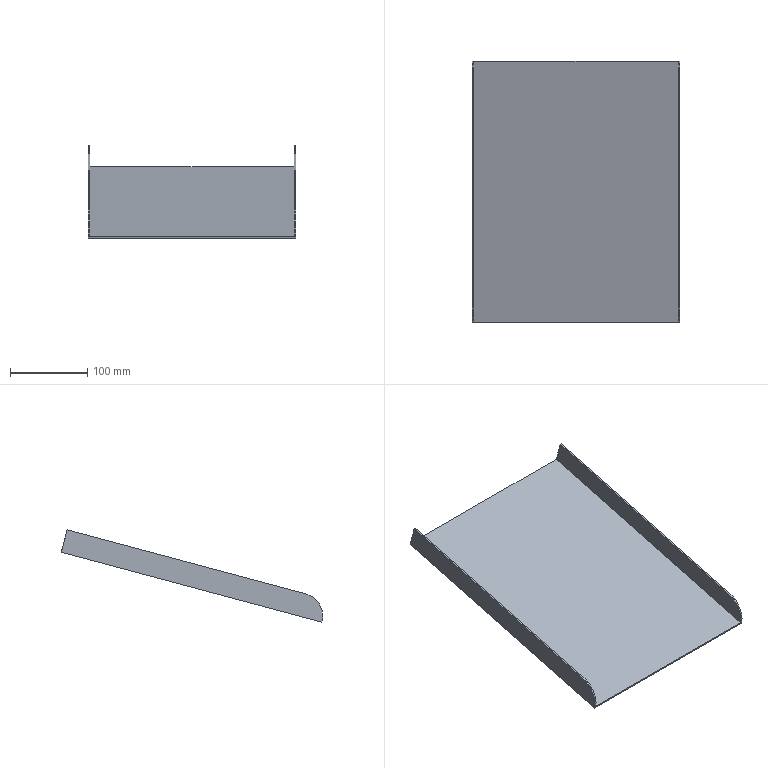Part | NX | features solid 2 | 1 solid | 12 faces | box 269.608 x 339.096 x 119.564 mm | volume 227153 mm3 | plane 10 | cylinder 2 | commonest cylinder face diameters 60 x2
STEP:
#1=CARTESIAN_POINT('',(378.,-610.733,-503.089));
#2=VERTEX_POINT('',#1);
#3=CARTESIAN_POINT('',(378.,-948.742,-593.658));
#4=VERTEX_POINT('',#3);
#5=CARTESIAN_POINT('',(378.,-784.599,-549.676));
#6=DIRECTION('',(0.,-0.9659,-0.2588));
#7=VECTOR('',#6,1000.);
#8=LINE('',#5,#7);
#9=EDGE_CURVE('',#2,#4,#8,.T.);
#10=ORIENTED_EDGE('',*,*,#9,.F.);
#11=CARTESIAN_POINT('',(112.392,-610.733,-503.089));
#12=VERTEX_POINT('',#11);
#13=CARTESIAN_POINT('',(378.,-610.733,-503.089));
#14=DIRECTION('',(1.,0.,0.));
#15=VECTOR('',#14,1000.);
#16=LINE('',#13,#15);
#17=EDGE_CURVE('',#2,#12,#16,.F.);
#18=ORIENTED_EDGE('',*,*,#17,.T.);
#19=CARTESIAN_POINT('',(112.392,-948.742,-593.658));
#20=VERTEX_POINT('',#19);
#21=CARTESIAN_POINT('',(112.392,-766.757,-544.895));
#22=DIRECTION('',(0.,0.9659,0.2588));
#23=VECTOR('',#22,1000.);
#24=LINE('',#21,#23);
#25=EDGE_CURVE('',#12,#20,#24,.F.);
#26=ORIENTED_EDGE('',*,*,#25,.T.);
#27=CARTESIAN_POINT('',(110.392,-948.742,-593.658));
#28=VERTEX_POINT('',#27);
#29=CARTESIAN_POINT('',(154.206,-948.742,-593.658));
#30=DIRECTION('',(-1.,0.,0.));
#31=VECTOR('',#30,1000.);
#32=LINE('',#29,#31);
#33=EDGE_CURVE('',#28,#20,#32,.F.);
#34=ORIENTED_EDGE('',*,*,#33,.F.);
#35=CARTESIAN_POINT('',(110.392,-948.807,-593.675));
#36=VERTEX_POINT('',#35);
#37=CARTESIAN_POINT('',(110.392,-795.624,-552.63));
#38=DIRECTION('',(0.,0.9659,0.2588));
#39=VECTOR('',#38,1000.);
#40=LINE('',#37,#39);
#41=EDGE_CURVE('',#28,#36,#40,.F.);
#42=ORIENTED_EDGE('',*,*,#41,.T.);
#43=CARTESIAN_POINT('',(380.,-948.807,-593.675));
#44=VERTEX_POINT('',#43);
#45=CARTESIAN_POINT('',(378.,-948.807,-593.675));
#46=DIRECTION('',(1.,0.,0.));
#47=VECTOR('',#46,1000.);
#48=LINE('',#45,#47);
#49=EDGE_CURVE('',#44,#36,#48,.F.);
#50=ORIENTED_EDGE('',*,*,#49,.F.);
#51=CARTESIAN_POINT('',(380.,-948.742,-593.658));
#52=VERTEX_POINT('',#51);
#53=CARTESIAN_POINT('',(380.,-784.599,-549.676));
#54=DIRECTION('',(0.,-0.9659,-0.2588));
#55=VECTOR('',#54,1000.);
#56=LINE('',#53,#55);
#57=EDGE_CURVE('',#52,#44,#56,.T.);
#58=ORIENTED_EDGE('',*,*,#57,.F.);
#59=CARTESIAN_POINT('',(390.,-948.742,-593.658));
#60=DIRECTION('',(1.,0.,0.));
#61=VECTOR('',#60,1000.);
#62=LINE('',#59,#61);
#63=EDGE_CURVE('',#4,#52,#62,.T.);
#64=ORIENTED_EDGE('',*,*,#63,.F.);
#65=EDGE_LOOP('',(#10,#18,#26,#34,#42,#50,#58,#64));
#66=FACE_BOUND('',#65,.T.);
#67=CARTESIAN_POINT('',(378.,-784.599,-549.676));
#68=DIRECTION('',(0.,-0.2588,0.9659));
#69=DIRECTION('',(1.,0.,0.));
#70=AXIS2_PLACEMENT_3D('',#67,#68,#69);
#71=PLANE('',#70);
#72=ADVANCED_FACE('',(#66),#71,.T.);
#73=ORIENTED_EDGE('',*,*,#17,.F.);
#74=CARTESIAN_POINT('',(378.,-617.98,-476.043));
#75=VERTEX_POINT('',#74);
#76=CARTESIAN_POINT('',(378.,-610.215,-505.021));
#77=DIRECTION('',(0.,0.2588,-0.9659));
#78=VECTOR('',#77,1000.);
#79=LINE('',#76,#78);
#80=EDGE_CURVE('',#2,#75,#79,.F.);
#81=ORIENTED_EDGE('',*,*,#80,.T.);
#82=CARTESIAN_POINT('',(380.,-617.98,-476.043));
#83=VERTEX_POINT('',#82);
#84=CARTESIAN_POINT('',(378.,-617.98,-476.043));
#85=DIRECTION('',(-1.,0.,0.));
#86=VECTOR('',#85,1000.);
#87=LINE('',#84,#86);
#88=EDGE_CURVE('',#83,#75,#87,.T.);
#89=ORIENTED_EDGE('',*,*,#88,.F.);
#90=CARTESIAN_POINT('',(380.,-610.215,-505.021));
#91=VERTEX_POINT('',#90);
#92=CARTESIAN_POINT('',(380.,-610.215,-505.021));
#93=DIRECTION('',(0.,0.2588,-0.9659));
#94=VECTOR('',#93,1000.);
#95=LINE('',#92,#94);
#96=EDGE_CURVE('',#91,#83,#95,.F.);
#97=ORIENTED_EDGE('',*,*,#96,.F.);
#98=CARTESIAN_POINT('',(110.392,-610.215,-505.021));
#99=VERTEX_POINT('',#98);
#100=CARTESIAN_POINT('',(378.,-610.215,-505.021));
#101=DIRECTION('',(1.,0.,0.));
#102=VECTOR('',#101,1000.);
#103=LINE('',#100,#102);
#104=EDGE_CURVE('',#91,#99,#103,.F.);
#105=ORIENTED_EDGE('',*,*,#104,.T.);
#106=CARTESIAN_POINT('',(110.392,-617.98,-476.043));
#107=VERTEX_POINT('',#106);
#108=CARTESIAN_POINT('',(110.392,-610.215,-505.021));
#109=DIRECTION('',(0.,-0.2588,0.9659));
#110=VECTOR('',#109,1000.);
#111=LINE('',#108,#110);
#112=EDGE_CURVE('',#99,#107,#111,.T.);
#113=ORIENTED_EDGE('',*,*,#112,.T.);
#114=CARTESIAN_POINT('',(112.392,-617.98,-476.043));
#115=VERTEX_POINT('',#114);
#116=CARTESIAN_POINT('',(378.,-617.98,-476.043));
#117=DIRECTION('',(-1.,0.,0.));
#118=VECTOR('',#117,1000.);
#119=LINE('',#116,#118);
#120=EDGE_CURVE('',#107,#115,#119,.F.);
#121=ORIENTED_EDGE('',*,*,#120,.T.);
#122=CARTESIAN_POINT('',(112.392,-610.215,-505.021));
#123=DIRECTION('',(0.,-0.2588,0.9659));
#124=VECTOR('',#123,1000.);
#125=LINE('',#122,#124);
#126=EDGE_CURVE('',#12,#115,#125,.T.);
#127=ORIENTED_EDGE('',*,*,#126,.F.);
#128=EDGE_LOOP('',(#73,#81,#89,#97,#105,#113,#121,#127));
#129=FACE_BOUND('',#128,.T.);
#130=CARTESIAN_POINT('',(378.,-610.215,-505.021));
#131=DIRECTION('',(0.,0.9659,0.2588));
#132=DIRECTION('',(-1.,0.,0.));
#133=AXIS2_PLACEMENT_3D('',#130,#131,#132);
#134=PLANE('',#133);
#135=ADVANCED_FACE('',(#129),#134,.T.);
#136=CARTESIAN_POINT('',(380.,-948.289,-595.607));
#137=VERTEX_POINT('',#136);
#138=CARTESIAN_POINT('',(380.,-948.289,-595.607));
#139=DIRECTION('',(0.,-0.2588,0.9659));
#140=VECTOR('',#139,1000.);
#141=LINE('',#138,#140);
#142=EDGE_CURVE('',#137,#44,#141,.T.);
#143=ORIENTED_EDGE('',*,*,#142,.F.);
#144=CARTESIAN_POINT('',(380.,-784.082,-551.608));
#145=DIRECTION('',(0.,-0.9659,-0.2588));
#146=VECTOR('',#145,1000.);
#147=LINE('',#144,#146);
#148=EDGE_CURVE('',#91,#137,#147,.T.);
#149=ORIENTED_EDGE('',*,*,#148,.F.);
#150=ORIENTED_EDGE('',*,*,#96,.T.);
#151=CARTESIAN_POINT('',(380.,-927.076,-558.865));
#152=VERTEX_POINT('',#151);
#153=CARTESIAN_POINT('',(380.,-791.846,-522.63));
#154=DIRECTION('',(0.,0.9659,0.2588));
#155=VECTOR('',#154,1000.);
#156=LINE('',#153,#155);
#157=EDGE_CURVE('',#83,#152,#156,.F.);
#158=ORIENTED_EDGE('',*,*,#157,.T.);
#159=CARTESIAN_POINT('',(380.,-919.311,-587.843));
#160=DIRECTION('',(-1.,0.,0.));
#161=DIRECTION('',(0.,0.,1.));
#162=AXIS2_PLACEMENT_3D('',#159,#160,#161);
#163=CIRCLE('',#162,30.);
#164=EDGE_CURVE('',#152,#52,#163,.F.);
#165=ORIENTED_EDGE('',*,*,#164,.T.);
#166=ORIENTED_EDGE('',*,*,#57,.T.);
#167=EDGE_LOOP('',(#143,#149,#150,#158,#165,#166));
#168=FACE_BOUND('',#167,.T.);
#169=CARTESIAN_POINT('',(380.,-784.082,-551.608));
#170=DIRECTION('',(-1.,0.,0.));
#171=DIRECTION('',(0.,-0.9659,-0.2588));
#172=AXIS2_PLACEMENT_3D('',#169,#170,#171);
#173=PLANE('',#172);
#174=ADVANCED_FACE('',(#168),#173,.F.);
#175=ORIENTED_EDGE('',*,*,#142,.T.);
#176=ORIENTED_EDGE('',*,*,#49,.T.);
#177=CARTESIAN_POINT('',(110.392,-948.289,-595.607));
#178=VERTEX_POINT('',#177);
#179=CARTESIAN_POINT('',(110.392,-936.311,-640.312));
#180=DIRECTION('',(0.,0.2588,-0.9659));
#181=VECTOR('',#180,1000.);
#182=LINE('',#179,#181);
#183=EDGE_CURVE('',#178,#36,#182,.F.);
#184=ORIENTED_EDGE('',*,*,#183,.F.);
#185=CARTESIAN_POINT('',(378.,-948.289,-595.607));
#186=DIRECTION('',(-1.,0.,0.));
#187=VECTOR('',#186,1000.);
#188=LINE('',#185,#187);
#189=EDGE_CURVE('',#137,#178,#188,.T.);
#190=ORIENTED_EDGE('',*,*,#189,.F.);
#191=EDGE_LOOP('',(#175,#176,#184,#190));
#192=FACE_BOUND('',#191,.T.);
#193=CARTESIAN_POINT('',(378.,-948.289,-595.607));
#194=DIRECTION('',(0.,0.9659,0.2588));
#195=DIRECTION('',(-1.,0.,0.));
#196=AXIS2_PLACEMENT_3D('',#193,#194,#195);
#197=PLANE('',#196);
#198=ADVANCED_FACE('',(#192),#197,.F.);
#199=ORIENTED_EDGE('',*,*,#41,.F.);
#200=CARTESIAN_POINT('',(110.392,-927.076,-558.865));
#201=VERTEX_POINT('',#200);
#202=CARTESIAN_POINT('',(110.392,-919.311,-587.843));
#203=DIRECTION('',(-1.,0.,0.));
#204=DIRECTION('',(0.,0.,1.));
#205=AXIS2_PLACEMENT_3D('',#202,#203,#204);
#206=CIRCLE('',#205,30.);
#207=EDGE_CURVE('',#28,#201,#206,.T.);
#208=ORIENTED_EDGE('',*,*,#207,.T.);
#209=CARTESIAN_POINT('',(110.392,-791.846,-522.63));
#210=DIRECTION('',(0.,0.9659,0.2588));
#211=VECTOR('',#210,1000.);
#212=LINE('',#209,#211);
#213=EDGE_CURVE('',#107,#201,#212,.F.);
#214=ORIENTED_EDGE('',*,*,#213,.F.);
#215=ORIENTED_EDGE('',*,*,#112,.F.);
#216=CARTESIAN_POINT('',(110.392,-795.107,-554.562));
#217=DIRECTION('',(0.,0.9659,0.2588));
#218=VECTOR('',#217,1000.);
#219=LINE('',#216,#218);
#220=EDGE_CURVE('',#99,#178,#219,.F.);
#221=ORIENTED_EDGE('',*,*,#220,.T.);
#222=ORIENTED_EDGE('',*,*,#183,.T.);
#223=EDGE_LOOP('',(#199,#208,#214,#215,#221,#222));
#224=FACE_BOUND('',#223,.T.);
#225=CARTESIAN_POINT('',(110.392,-783.128,-599.267));
#226=DIRECTION('',(-1.,0.,0.));
#227=DIRECTION('',(0.,-0.9397,-0.342));
#228=AXIS2_PLACEMENT_3D('',#225,#226,#227);
#229=PLANE('',#228);
#230=ADVANCED_FACE('',(#224),#229,.T.);
#231=ORIENTED_EDGE('',*,*,#220,.F.);
#232=ORIENTED_EDGE('',*,*,#104,.F.);
#233=ORIENTED_EDGE('',*,*,#148,.T.);
#234=ORIENTED_EDGE('',*,*,#189,.T.);
#235=EDGE_LOOP('',(#231,#232,#233,#234));
#236=FACE_BOUND('',#235,.T.);
#237=CARTESIAN_POINT('',(378.,-784.082,-551.608));
#238=DIRECTION('',(0.,-0.2588,0.9659));
#239=DIRECTION('',(1.,0.,0.));
#240=AXIS2_PLACEMENT_3D('',#237,#238,#239);
#241=PLANE('',#240);
#242=ADVANCED_FACE('',(#236),#241,.F.);
#243=ORIENTED_EDGE('',*,*,#213,.T.);
#244=CARTESIAN_POINT('',(112.392,-927.076,-558.865));
#245=VERTEX_POINT('',#244);
#246=CARTESIAN_POINT('',(154.206,-927.076,-558.865));
#247=DIRECTION('',(-1.,0.,0.));
#248=VECTOR('',#247,1000.);
#249=LINE('',#246,#248);
#250=EDGE_CURVE('',#201,#245,#249,.F.);
#251=ORIENTED_EDGE('',*,*,#250,.T.);
#252=CARTESIAN_POINT('',(112.392,-791.846,-522.63));
#253=DIRECTION('',(0.,0.9659,0.2588));
#254=VECTOR('',#253,1000.);
#255=LINE('',#252,#254);
#256=EDGE_CURVE('',#115,#245,#255,.F.);
#257=ORIENTED_EDGE('',*,*,#256,.F.);
#258=ORIENTED_EDGE('',*,*,#120,.F.);
#259=EDGE_LOOP('',(#243,#251,#257,#258));
#260=FACE_BOUND('',#259,.T.);
#261=CARTESIAN_POINT('',(154.206,-791.846,-522.63));
#262=DIRECTION('',(0.,0.2588,-0.9659));
#263=DIRECTION('',(0.,-0.9659,-0.2588));
#264=AXIS2_PLACEMENT_3D('',#261,#262,#263);
#265=PLANE('',#264);
#266=ADVANCED_FACE('',(#260),#265,.F.);
#267=ORIENTED_EDGE('',*,*,#25,.F.);
#268=ORIENTED_EDGE('',*,*,#126,.T.);
#269=ORIENTED_EDGE('',*,*,#256,.T.);
#270=CARTESIAN_POINT('',(112.392,-919.311,-587.843));
#271=DIRECTION('',(-1.,0.,0.));
#272=DIRECTION('',(0.,0.,1.));
#273=AXIS2_PLACEMENT_3D('',#270,#271,#272);
#274=CIRCLE('',#273,30.);
#275=EDGE_CURVE('',#245,#20,#274,.F.);
#276=ORIENTED_EDGE('',*,*,#275,.T.);
#277=EDGE_LOOP('',(#267,#268,#269,#276));
#278=FACE_BOUND('',#277,.T.);
#279=CARTESIAN_POINT('',(112.392,-754.937,-589.006));
#280=DIRECTION('',(-1.,0.,0.));
#281=DIRECTION('',(0.,0.,1.));
#282=AXIS2_PLACEMENT_3D('',#279,#280,#281);
#283=PLANE('',#282);
#284=ADVANCED_FACE('',(#278),#283,.F.);
#285=ORIENTED_EDGE('',*,*,#207,.F.);
#286=ORIENTED_EDGE('',*,*,#33,.T.);
#287=ORIENTED_EDGE('',*,*,#275,.F.);
#288=ORIENTED_EDGE('',*,*,#250,.F.);
#289=EDGE_LOOP('',(#285,#286,#287,#288));
#290=FACE_BOUND('',#289,.T.);
#291=CARTESIAN_POINT('',(154.206,-919.311,-587.843));
#292=DIRECTION('',(-1.,0.,0.));
#293=DIRECTION('',(0.,-0.2588,0.9659));
#294=AXIS2_PLACEMENT_3D('',#291,#292,#293);
#295=CYLINDRICAL_SURFACE('',#294,30.);
#296=ADVANCED_FACE('',(#290),#295,.T.);
#297=CARTESIAN_POINT('',(378.,-927.076,-558.865));
#298=VERTEX_POINT('',#297);
#299=CARTESIAN_POINT('',(378.,-791.846,-522.63));
#300=DIRECTION('',(0.,0.9659,0.2588));
#301=VECTOR('',#300,1000.);
#302=LINE('',#299,#301);
#303=EDGE_CURVE('',#75,#298,#302,.F.);
#304=ORIENTED_EDGE('',*,*,#303,.T.);
#305=CARTESIAN_POINT('',(390.,-927.076,-558.865));
#306=DIRECTION('',(-1.,0.,0.));
#307=VECTOR('',#306,1000.);
#308=LINE('',#305,#307);
#309=EDGE_CURVE('',#298,#152,#308,.F.);
#310=ORIENTED_EDGE('',*,*,#309,.T.);
#311=ORIENTED_EDGE('',*,*,#157,.F.);
#312=ORIENTED_EDGE('',*,*,#88,.T.);
#313=EDGE_LOOP('',(#304,#310,#311,#312));
#314=FACE_BOUND('',#313,.T.);
#315=CARTESIAN_POINT('',(390.,-791.846,-522.63));
#316=DIRECTION('',(0.,0.2588,-0.9659));
#317=DIRECTION('',(0.,-0.9659,-0.2588));
#318=AXIS2_PLACEMENT_3D('',#315,#316,#317);
#319=PLANE('',#318);
#320=ADVANCED_FACE('',(#314),#319,.F.);
#321=ORIENTED_EDGE('',*,*,#80,.F.);
#322=ORIENTED_EDGE('',*,*,#9,.T.);
#323=CARTESIAN_POINT('',(378.,-919.311,-587.843));
#324=DIRECTION('',(-1.,0.,0.));
#325=DIRECTION('',(0.,0.,1.));
#326=AXIS2_PLACEMENT_3D('',#323,#324,#325);
#327=CIRCLE('',#326,30.);
#328=EDGE_CURVE('',#4,#298,#327,.T.);
#329=ORIENTED_EDGE('',*,*,#328,.T.);
#330=ORIENTED_EDGE('',*,*,#303,.F.);
#331=EDGE_LOOP('',(#321,#322,#329,#330));
#332=FACE_BOUND('',#331,.T.);
#333=CARTESIAN_POINT('',(378.,-784.082,-551.608));
#334=DIRECTION('',(-1.,0.,0.));
#335=DIRECTION('',(0.,-0.2588,0.9659));
#336=AXIS2_PLACEMENT_3D('',#333,#334,#335);
#337=PLANE('',#336);
#338=ADVANCED_FACE('',(#332),#337,.T.);
#339=ORIENTED_EDGE('',*,*,#328,.F.);
#340=ORIENTED_EDGE('',*,*,#63,.T.);
#341=ORIENTED_EDGE('',*,*,#164,.F.);
#342=ORIENTED_EDGE('',*,*,#309,.F.);
#343=EDGE_LOOP('',(#339,#340,#341,#342));
#344=FACE_BOUND('',#343,.T.);
#345=CARTESIAN_POINT('',(390.,-919.311,-587.843));
#346=DIRECTION('',(1.,0.,0.));
#347=DIRECTION('',(0.,0.2588,-0.9659));
#348=AXIS2_PLACEMENT_3D('',#345,#346,#347);
#349=CYLINDRICAL_SURFACE('',#348,30.);
#350=ADVANCED_FACE('',(#344),#349,.T.);
#351=CLOSED_SHELL('',(#72,#135,#174,#198,#230,#242,#266,#284,#296,#320,#338,#350));
#352=MANIFOLD_SOLID_BREP('',#351);
#353=(LENGTH_UNIT()NAMED_UNIT(*)SI_UNIT(.MILLI.,.METRE.));
#354=UNCERTAINTY_MEASURE_WITH_UNIT(LENGTH_MEASURE(0.00001),#353,'','');
#355=(NAMED_UNIT(*)PLANE_ANGLE_UNIT()SI_UNIT($,.RADIAN.));
#356=(NAMED_UNIT(*)SI_UNIT($,.STERADIAN.)SOLID_ANGLE_UNIT());
#357=(GEOMETRIC_REPRESENTATION_CONTEXT(3)GLOBAL_UNCERTAINTY_ASSIGNED_CONTEXT((#354))GLOBAL_UNIT_ASSIGNED_CONTEXT((#353,#355,#356))REPRESENTATION_CONTEXT('',''));
#358=ADVANCED_BREP_SHAPE_REPRESENTATION('',(#352),#357);